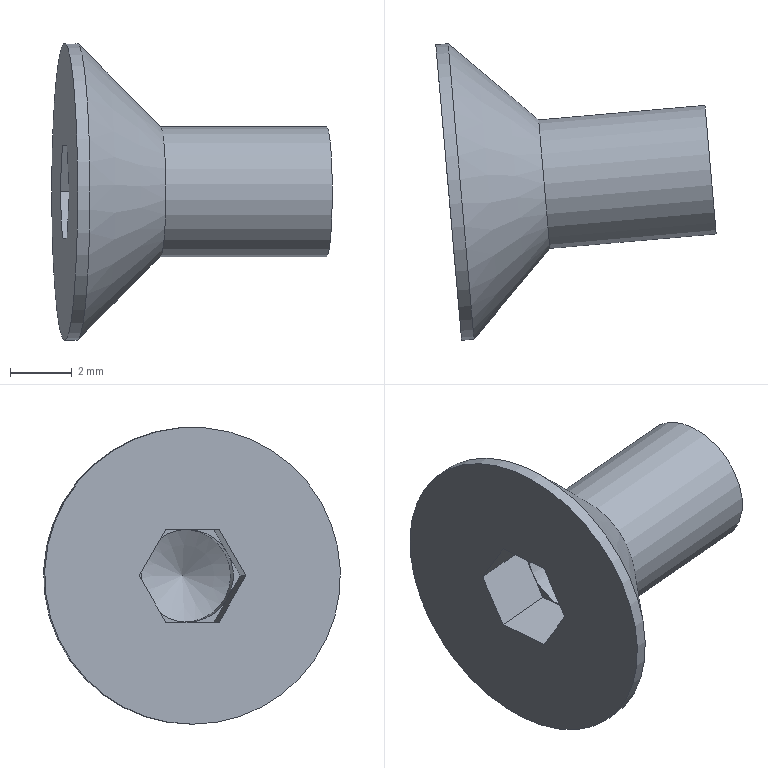Part | NX | features 4 2 | 1 solid | 19 faces | box 9.069 x 9.598 x 9.6 mm | volume 185.183 mm3 | plane 14 | cylinder 3 | cone 2 | commonest cylinder face diameters 3 x1 4.2 x1 9.6 x1
STEP:
#1=CARTESIAN_POINT('',(730.589,495.561,-274.75));
#2=VERTEX_POINT('',#1);
#3=CARTESIAN_POINT('',(730.589,495.561,-273.25));
#4=DIRECTION('',(0.9962,0.08716,0.));
#5=DIRECTION('',(0.,0.,-1.));
#6=AXIS2_PLACEMENT_3D('',#3,#4,#5);
#7=CIRCLE('',#6,1.5);
#8=EDGE_CURVE('',#2,#2,#7,.T.);
#9=ORIENTED_EDGE('',*,*,#8,.F.);
#10=EDGE_LOOP('',(#9));
#11=FACE_BOUND('',#10,.T.);
#12=CARTESIAN_POINT('',(731.452,495.636,-273.25));
#13=VERTEX_POINT('',#12);
#14=VERTEX_LOOP('',#13);
#15=FACE_BOUND('',#14,.T.);
#16=CARTESIAN_POINT('',(731.021,495.599,-273.25));
#17=DIRECTION('',(-0.9962,-0.08716,0.));
#18=DIRECTION('',(0.08716,-0.9962,0.));
#19=AXIS2_PLACEMENT_3D('',#16,#17,#18);
#20=CONICAL_SURFACE('',#19,0.75,1.047);
#21=ADVANCED_FACE('',(#11,#15),#20,.F.);
#22=ORIENTED_EDGE('',*,*,#8,.T.);
#23=EDGE_LOOP('',(#22));
#24=FACE_BOUND('',#23,.T.);
#25=CARTESIAN_POINT('',(729.706,494.18,-274.));
#26=VERTEX_POINT('',#25);
#27=CARTESIAN_POINT('',(729.593,495.474,-274.75));
#28=VERTEX_POINT('',#27);
#29=CARTESIAN_POINT('',(729.593,495.474,-273.25));
#30=DIRECTION('',(0.9962,0.08716,0.));
#31=DIRECTION('',(0.,0.,-1.));
#32=AXIS2_PLACEMENT_3D('',#29,#30,#31);
#33=CIRCLE('',#32,1.5);
#34=EDGE_CURVE('',#26,#28,#33,.T.);
#35=ORIENTED_EDGE('',*,*,#34,.F.);
#36=CARTESIAN_POINT('',(729.706,494.18,-272.5));
#37=VERTEX_POINT('',#36);
#38=CARTESIAN_POINT('',(729.593,495.474,-273.25));
#39=DIRECTION('',(0.9962,0.08716,0.));
#40=DIRECTION('',(0.,0.,-1.));
#41=AXIS2_PLACEMENT_3D('',#38,#39,#40);
#42=CIRCLE('',#41,1.5);
#43=EDGE_CURVE('',#37,#26,#42,.T.);
#44=ORIENTED_EDGE('',*,*,#43,.F.);
#45=CARTESIAN_POINT('',(729.593,495.474,-271.75));
#46=VERTEX_POINT('',#45);
#47=CARTESIAN_POINT('',(729.593,495.474,-273.25));
#48=DIRECTION('',(0.9962,0.08716,0.));
#49=DIRECTION('',(0.,0.,-1.));
#50=AXIS2_PLACEMENT_3D('',#47,#48,#49);
#51=CIRCLE('',#50,1.5);
#52=EDGE_CURVE('',#46,#37,#51,.T.);
#53=ORIENTED_EDGE('',*,*,#52,.F.);
#54=CARTESIAN_POINT('',(729.48,496.768,-272.5));
#55=VERTEX_POINT('',#54);
#56=CARTESIAN_POINT('',(729.593,495.474,-273.25));
#57=DIRECTION('',(0.9962,0.08716,0.));
#58=DIRECTION('',(0.,0.,-1.));
#59=AXIS2_PLACEMENT_3D('',#56,#57,#58);
#60=CIRCLE('',#59,1.5);
#61=EDGE_CURVE('',#55,#46,#60,.T.);
#62=ORIENTED_EDGE('',*,*,#61,.F.);
#63=CARTESIAN_POINT('',(729.48,496.768,-274.));
#64=VERTEX_POINT('',#63);
#65=CARTESIAN_POINT('',(729.593,495.474,-273.25));
#66=DIRECTION('',(0.9962,0.08716,0.));
#67=DIRECTION('',(0.,0.,-1.));
#68=AXIS2_PLACEMENT_3D('',#65,#66,#67);
#69=CIRCLE('',#68,1.5);
#70=EDGE_CURVE('',#64,#55,#69,.T.);
#71=ORIENTED_EDGE('',*,*,#70,.F.);
#72=CARTESIAN_POINT('',(729.593,495.474,-273.25));
#73=DIRECTION('',(0.9962,0.08716,0.));
#74=DIRECTION('',(0.,0.,-1.));
#75=AXIS2_PLACEMENT_3D('',#72,#73,#74);
#76=CIRCLE('',#75,1.5);
#77=EDGE_CURVE('',#28,#64,#76,.T.);
#78=ORIENTED_EDGE('',*,*,#77,.F.);
#79=EDGE_LOOP('',(#35,#44,#53,#62,#71,#78));
#80=FACE_BOUND('',#79,.T.);
#81=CARTESIAN_POINT('',(729.095,495.43,-273.25));
#82=DIRECTION('',(0.9962,0.08716,0.));
#83=DIRECTION('',(-0.08716,0.9962,0.));
#84=AXIS2_PLACEMENT_3D('',#81,#82,#83);
#85=CYLINDRICAL_SURFACE('',#84,1.5);
#86=ADVANCED_FACE('',(#24,#80),#85,.F.);
#87=CARTESIAN_POINT('',(727.999,495.334,-278.05));
#88=VERTEX_POINT('',#87);
#89=CARTESIAN_POINT('',(727.999,495.334,-273.25));
#90=DIRECTION('',(0.9962,0.08716,0.));
#91=DIRECTION('',(0.,0.,-1.));
#92=AXIS2_PLACEMENT_3D('',#89,#90,#91);
#93=CIRCLE('',#92,4.8);
#94=EDGE_CURVE('',#88,#88,#93,.T.);
#95=ORIENTED_EDGE('',*,*,#94,.F.);
#96=EDGE_LOOP('',(#95));
#97=FACE_BOUND('',#96,.T.);
#98=CARTESIAN_POINT('',(727.601,495.299,-278.05));
#99=VERTEX_POINT('',#98);
#100=CARTESIAN_POINT('',(727.601,495.299,-273.25));
#101=DIRECTION('',(0.9962,0.08716,0.));
#102=DIRECTION('',(0.,0.,-1.));
#103=AXIS2_PLACEMENT_3D('',#100,#101,#102);
#104=CIRCLE('',#103,4.8);
#105=EDGE_CURVE('',#99,#99,#104,.T.);
#106=ORIENTED_EDGE('',*,*,#105,.T.);
#107=EDGE_LOOP('',(#106));
#108=FACE_BOUND('',#107,.T.);
#109=CARTESIAN_POINT('',(727.8,495.317,-273.25));
#110=DIRECTION('',(0.9962,0.08716,0.));
#111=DIRECTION('',(-0.08716,0.9962,0.));
#112=AXIS2_PLACEMENT_3D('',#109,#110,#111);
#113=CYLINDRICAL_SURFACE('',#112,4.8);
#114=ADVANCED_FACE('',(#97,#108),#113,.T.);
#115=CARTESIAN_POINT('',(730.689,495.57,-275.35));
#116=VERTEX_POINT('',#115);
#117=CARTESIAN_POINT('',(730.689,495.57,-273.25));
#118=DIRECTION('',(0.9962,0.08716,0.));
#119=DIRECTION('',(0.,0.,-1.));
#120=AXIS2_PLACEMENT_3D('',#117,#118,#119);
#121=CIRCLE('',#120,2.1);
#122=EDGE_CURVE('',#116,#116,#121,.T.);
#123=ORIENTED_EDGE('',*,*,#122,.F.);
#124=EDGE_LOOP('',(#123));
#125=FACE_BOUND('',#124,.T.);
#126=ORIENTED_EDGE('',*,*,#94,.T.);
#127=EDGE_LOOP('',(#126));
#128=FACE_BOUND('',#127,.T.);
#129=CARTESIAN_POINT('',(729.344,495.452,-273.25));
#130=DIRECTION('',(-0.9962,-0.08716,0.));
#131=DIRECTION('',(0.08716,-0.9962,0.));
#132=AXIS2_PLACEMENT_3D('',#129,#130,#131);
#133=CONICAL_SURFACE('',#132,3.45,0.7854);
#134=ADVANCED_FACE('',(#125,#128),#133,.T.);
#135=CARTESIAN_POINT('',(736.068,496.04,-275.35));
#136=VERTEX_POINT('',#135);
#137=CARTESIAN_POINT('',(736.068,496.04,-273.25));
#138=DIRECTION('',(0.9962,0.08716,0.));
#139=DIRECTION('',(0.,0.,-1.));
#140=AXIS2_PLACEMENT_3D('',#137,#138,#139);
#141=CIRCLE('',#140,2.1);
#142=EDGE_CURVE('',#136,#136,#141,.T.);
#143=ORIENTED_EDGE('',*,*,#142,.F.);
#144=EDGE_LOOP('',(#143));
#145=FACE_BOUND('',#144,.T.);
#146=ORIENTED_EDGE('',*,*,#122,.T.);
#147=EDGE_LOOP('',(#146));
#148=FACE_BOUND('',#147,.T.);
#149=CARTESIAN_POINT('',(733.378,495.805,-273.25));
#150=DIRECTION('',(0.9962,0.08716,0.));
#151=DIRECTION('',(-0.08716,0.9962,0.));
#152=AXIS2_PLACEMENT_3D('',#149,#150,#151);
#153=CYLINDRICAL_SURFACE('',#152,2.1);
#154=ADVANCED_FACE('',(#145,#148),#153,.T.);
#155=CARTESIAN_POINT('',(727.676,494.437,-274.75));
#156=VERTEX_POINT('',#155);
#157=CARTESIAN_POINT('',(727.752,493.574,-273.25));
#158=VERTEX_POINT('',#157);
#159=CARTESIAN_POINT('',(727.673,494.469,-274.806));
#160=DIRECTION('',(0.04358,-0.4981,0.866));
#161=VECTOR('',#160,1000.);
#162=LINE('',#159,#161);
#163=EDGE_CURVE('',#156,#158,#162,.T.);
#164=ORIENTED_EDGE('',*,*,#163,.T.);
#165=CARTESIAN_POINT('',(729.744,493.748,-273.25));
#166=VERTEX_POINT('',#165);
#167=CARTESIAN_POINT('',(725.759,493.4,-273.25));
#168=DIRECTION('',(0.9962,0.08716,0.));
#169=VECTOR('',#168,1000.);
#170=LINE('',#167,#169);
#171=EDGE_CURVE('',#158,#166,#170,.T.);
#172=ORIENTED_EDGE('',*,*,#171,.T.);
#173=CARTESIAN_POINT('',(729.744,493.748,-273.25));
#174=DIRECTION('',(-0.04358,0.4981,-0.866));
#175=VECTOR('',#174,1000.);
#176=LINE('',#173,#175);
#177=EDGE_CURVE('',#166,#26,#176,.T.);
#178=ORIENTED_EDGE('',*,*,#177,.T.);
#179=CARTESIAN_POINT('',(729.668,494.611,-274.75));
#180=VERTEX_POINT('',#179);
#181=CARTESIAN_POINT('',(729.744,493.748,-273.25));
#182=DIRECTION('',(-0.04358,0.4981,-0.866));
#183=VECTOR('',#182,1000.);
#184=LINE('',#181,#183);
#185=EDGE_CURVE('',#26,#180,#184,.T.);
#186=ORIENTED_EDGE('',*,*,#185,.T.);
#187=CARTESIAN_POINT('',(725.684,494.262,-274.75));
#188=DIRECTION('',(0.9962,0.08716,0.));
#189=VECTOR('',#188,1000.);
#190=LINE('',#187,#189);
#191=EDGE_CURVE('',#156,#180,#190,.T.);
#192=ORIENTED_EDGE('',*,*,#191,.F.);
#193=EDGE_LOOP('',(#164,#172,#178,#186,#192));
#194=FACE_BOUND('',#193,.T.);
#195=CARTESIAN_POINT('',(725.759,493.4,-273.25));
#196=DIRECTION('',(0.07548,-0.8627,-0.5));
#197=DIRECTION('',(-0.04358,0.4981,-0.866));
#198=AXIS2_PLACEMENT_3D('',#195,#196,#197);
#199=PLANE('',#198);
#200=ADVANCED_FACE('',(#194),#199,.F.);
#201=CARTESIAN_POINT('',(727.525,496.162,-274.75));
#202=VERTEX_POINT('',#201);
#203=CARTESIAN_POINT('',(727.638,494.868,-274.75));
#204=DIRECTION('',(0.08716,-0.9962,0.));
#205=VECTOR('',#204,1000.);
#206=LINE('',#203,#205);
#207=EDGE_CURVE('',#202,#156,#206,.T.);
#208=ORIENTED_EDGE('',*,*,#207,.T.);
#209=ORIENTED_EDGE('',*,*,#191,.T.);
#210=CARTESIAN_POINT('',(729.668,494.611,-274.75));
#211=DIRECTION('',(-0.08716,0.9962,0.));
#212=VECTOR('',#211,1000.);
#213=LINE('',#210,#212);
#214=EDGE_CURVE('',#180,#28,#213,.T.);
#215=ORIENTED_EDGE('',*,*,#214,.T.);
#216=CARTESIAN_POINT('',(729.517,496.336,-274.75));
#217=VERTEX_POINT('',#216);
#218=CARTESIAN_POINT('',(729.668,494.611,-274.75));
#219=DIRECTION('',(-0.08716,0.9962,0.));
#220=VECTOR('',#219,1000.);
#221=LINE('',#218,#220);
#222=EDGE_CURVE('',#28,#217,#221,.T.);
#223=ORIENTED_EDGE('',*,*,#222,.T.);
#224=CARTESIAN_POINT('',(725.533,495.988,-274.75));
#225=DIRECTION('',(0.9962,0.08716,0.));
#226=VECTOR('',#225,1000.);
#227=LINE('',#224,#226);
#228=EDGE_CURVE('',#202,#217,#227,.T.);
#229=ORIENTED_EDGE('',*,*,#228,.F.);
#230=EDGE_LOOP('',(#208,#209,#215,#223,#229));
#231=FACE_BOUND('',#230,.T.);
#232=CARTESIAN_POINT('',(725.684,494.262,-274.75));
#233=DIRECTION('',(0.,0.,-1.));
#234=DIRECTION('',(-0.9962,-0.08716,0.));
#235=AXIS2_PLACEMENT_3D('',#232,#233,#234);
#236=PLANE('',#235);
#237=ADVANCED_FACE('',(#231),#236,.F.);
#238=CARTESIAN_POINT('',(727.676,494.437,-271.75));
#239=VERTEX_POINT('',#238);
#240=CARTESIAN_POINT('',(727.754,493.542,-273.306));
#241=DIRECTION('',(-0.04358,0.4981,0.866));
#242=VECTOR('',#241,1000.);
#243=LINE('',#240,#242);
#244=EDGE_CURVE('',#158,#239,#243,.T.);
#245=ORIENTED_EDGE('',*,*,#244,.T.);
#246=CARTESIAN_POINT('',(729.668,494.611,-271.75));
#247=VERTEX_POINT('',#246);
#248=CARTESIAN_POINT('',(725.684,494.262,-271.75));
#249=DIRECTION('',(0.9962,0.08716,0.));
#250=VECTOR('',#249,1000.);
#251=LINE('',#248,#250);
#252=EDGE_CURVE('',#239,#247,#251,.T.);
#253=ORIENTED_EDGE('',*,*,#252,.T.);
#254=CARTESIAN_POINT('',(729.668,494.611,-271.75));
#255=DIRECTION('',(0.04358,-0.4981,-0.866));
#256=VECTOR('',#255,1000.);
#257=LINE('',#254,#256);
#258=EDGE_CURVE('',#247,#37,#257,.T.);
#259=ORIENTED_EDGE('',*,*,#258,.T.);
#260=CARTESIAN_POINT('',(729.668,494.611,-271.75));
#261=DIRECTION('',(0.04358,-0.4981,-0.866));
#262=VECTOR('',#261,1000.);
#263=LINE('',#260,#262);
#264=EDGE_CURVE('',#37,#166,#263,.T.);
#265=ORIENTED_EDGE('',*,*,#264,.T.);
#266=ORIENTED_EDGE('',*,*,#171,.F.);
#267=EDGE_LOOP('',(#245,#253,#259,#265,#266));
#268=FACE_BOUND('',#267,.T.);
#269=CARTESIAN_POINT('',(725.684,494.262,-271.75));
#270=DIRECTION('',(0.07548,-0.8627,0.5));
#271=DIRECTION('',(0.04358,-0.4981,-0.866));
#272=AXIS2_PLACEMENT_3D('',#269,#270,#271);
#273=PLANE('',#272);
#274=ADVANCED_FACE('',(#268),#273,.F.);
#275=CARTESIAN_POINT('',(727.45,497.025,-273.25));
#276=VERTEX_POINT('',#275);
#277=CARTESIAN_POINT('',(727.566,495.698,-275.556));
#278=DIRECTION('',(0.04358,-0.4981,-0.866));
#279=VECTOR('',#278,1000.);
#280=LINE('',#277,#279);
#281=EDGE_CURVE('',#276,#202,#280,.T.);
#282=ORIENTED_EDGE('',*,*,#281,.T.);
#283=ORIENTED_EDGE('',*,*,#228,.T.);
#284=CARTESIAN_POINT('',(729.517,496.336,-274.75));
#285=DIRECTION('',(-0.04358,0.4981,0.866));
#286=VECTOR('',#285,1000.);
#287=LINE('',#284,#286);
#288=EDGE_CURVE('',#217,#64,#287,.T.);
#289=ORIENTED_EDGE('',*,*,#288,.T.);
#290=CARTESIAN_POINT('',(729.442,497.199,-273.25));
#291=VERTEX_POINT('',#290);
#292=CARTESIAN_POINT('',(729.517,496.336,-274.75));
#293=DIRECTION('',(-0.04358,0.4981,0.866));
#294=VECTOR('',#293,1000.);
#295=LINE('',#292,#294);
#296=EDGE_CURVE('',#64,#291,#295,.T.);
#297=ORIENTED_EDGE('',*,*,#296,.T.);
#298=CARTESIAN_POINT('',(725.457,496.85,-273.25));
#299=DIRECTION('',(0.9962,0.08716,0.));
#300=VECTOR('',#299,1000.);
#301=LINE('',#298,#300);
#302=EDGE_CURVE('',#276,#291,#301,.T.);
#303=ORIENTED_EDGE('',*,*,#302,.F.);
#304=EDGE_LOOP('',(#282,#283,#289,#297,#303));
#305=FACE_BOUND('',#304,.T.);
#306=CARTESIAN_POINT('',(725.533,495.988,-274.75));
#307=DIRECTION('',(-0.07548,0.8627,-0.5));
#308=DIRECTION('',(-0.04358,0.4981,0.866));
#309=AXIS2_PLACEMENT_3D('',#306,#307,#308);
#310=PLANE('',#309);
#311=ADVANCED_FACE('',(#305),#310,.F.);
#312=ORIENTED_EDGE('',*,*,#61,.T.);
#313=CARTESIAN_POINT('',(729.517,496.336,-271.75));
#314=VERTEX_POINT('',#313);
#315=CARTESIAN_POINT('',(729.517,496.336,-271.75));
#316=DIRECTION('',(0.08716,-0.9962,0.));
#317=VECTOR('',#316,1000.);
#318=LINE('',#315,#317);
#319=EDGE_CURVE('',#314,#46,#318,.T.);
#320=ORIENTED_EDGE('',*,*,#319,.F.);
#321=CARTESIAN_POINT('',(729.442,497.199,-273.25));
#322=DIRECTION('',(0.04358,-0.4981,0.866));
#323=VECTOR('',#322,1000.);
#324=LINE('',#321,#323);
#325=EDGE_CURVE('',#55,#314,#324,.T.);
#326=ORIENTED_EDGE('',*,*,#325,.F.);
#327=EDGE_LOOP('',(#312,#320,#326));
#328=FACE_BOUND('',#327,.T.);
#329=CARTESIAN_POINT('',(729.593,495.474,-273.25));
#330=DIRECTION('',(-0.9962,-0.08716,0.));
#331=DIRECTION('',(0.08716,-0.9962,0.));
#332=AXIS2_PLACEMENT_3D('',#329,#330,#331);
#333=PLANE('',#332);
#334=ADVANCED_FACE('',(#328),#333,.T.);
#335=ORIENTED_EDGE('',*,*,#52,.T.);
#336=ORIENTED_EDGE('',*,*,#258,.F.);
#337=CARTESIAN_POINT('',(729.517,496.336,-271.75));
#338=DIRECTION('',(0.08716,-0.9962,0.));
#339=VECTOR('',#338,1000.);
#340=LINE('',#337,#339);
#341=EDGE_CURVE('',#46,#247,#340,.T.);
#342=ORIENTED_EDGE('',*,*,#341,.F.);
#343=EDGE_LOOP('',(#335,#336,#342));
#344=FACE_BOUND('',#343,.T.);
#345=CARTESIAN_POINT('',(729.593,495.474,-273.25));
#346=DIRECTION('',(-0.9962,-0.08716,0.));
#347=DIRECTION('',(0.08716,-0.9962,0.));
#348=AXIS2_PLACEMENT_3D('',#345,#346,#347);
#349=PLANE('',#348);
#350=ADVANCED_FACE('',(#344),#349,.T.);
#351=ORIENTED_EDGE('',*,*,#43,.T.);
#352=ORIENTED_EDGE('',*,*,#177,.F.);
#353=ORIENTED_EDGE('',*,*,#264,.F.);
#354=EDGE_LOOP('',(#351,#352,#353));
#355=FACE_BOUND('',#354,.T.);
#356=CARTESIAN_POINT('',(729.593,495.474,-273.25));
#357=DIRECTION('',(-0.9962,-0.08716,0.));
#358=DIRECTION('',(0.08716,-0.9962,0.));
#359=AXIS2_PLACEMENT_3D('',#356,#357,#358);
#360=PLANE('',#359);
#361=ADVANCED_FACE('',(#355),#360,.T.);
#362=ORIENTED_EDGE('',*,*,#34,.T.);
#363=ORIENTED_EDGE('',*,*,#214,.F.);
#364=ORIENTED_EDGE('',*,*,#185,.F.);
#365=EDGE_LOOP('',(#362,#363,#364));
#366=FACE_BOUND('',#365,.T.);
#367=CARTESIAN_POINT('',(729.593,495.474,-273.25));
#368=DIRECTION('',(-0.9962,-0.08716,0.));
#369=DIRECTION('',(0.08716,-0.9962,0.));
#370=AXIS2_PLACEMENT_3D('',#367,#368,#369);
#371=PLANE('',#370);
#372=ADVANCED_FACE('',(#366),#371,.T.);
#373=ORIENTED_EDGE('',*,*,#77,.T.);
#374=ORIENTED_EDGE('',*,*,#288,.F.);
#375=ORIENTED_EDGE('',*,*,#222,.F.);
#376=EDGE_LOOP('',(#373,#374,#375));
#377=FACE_BOUND('',#376,.T.);
#378=CARTESIAN_POINT('',(729.593,495.474,-273.25));
#379=DIRECTION('',(-0.9962,-0.08716,0.));
#380=DIRECTION('',(0.08716,-0.9962,0.));
#381=AXIS2_PLACEMENT_3D('',#378,#379,#380);
#382=PLANE('',#381);
#383=ADVANCED_FACE('',(#377),#382,.T.);
#384=ORIENTED_EDGE('',*,*,#70,.T.);
#385=CARTESIAN_POINT('',(729.442,497.199,-273.25));
#386=DIRECTION('',(0.04358,-0.4981,0.866));
#387=VECTOR('',#386,1000.);
#388=LINE('',#385,#387);
#389=EDGE_CURVE('',#291,#55,#388,.T.);
#390=ORIENTED_EDGE('',*,*,#389,.F.);
#391=ORIENTED_EDGE('',*,*,#296,.F.);
#392=EDGE_LOOP('',(#384,#390,#391));
#393=FACE_BOUND('',#392,.T.);
#394=CARTESIAN_POINT('',(729.593,495.474,-273.25));
#395=DIRECTION('',(-0.9962,-0.08716,0.));
#396=DIRECTION('',(0.08716,-0.9962,0.));
#397=AXIS2_PLACEMENT_3D('',#394,#395,#396);
#398=PLANE('',#397);
#399=ADVANCED_FACE('',(#393),#398,.T.);
#400=CARTESIAN_POINT('',(727.525,496.162,-271.75));
#401=VERTEX_POINT('',#400);
#402=CARTESIAN_POINT('',(727.563,495.731,-271.75));
#403=DIRECTION('',(-0.08716,0.9962,0.));
#404=VECTOR('',#403,1000.);
#405=LINE('',#402,#404);
#406=EDGE_CURVE('',#239,#401,#405,.T.);
#407=ORIENTED_EDGE('',*,*,#406,.T.);
#408=CARTESIAN_POINT('',(725.533,495.988,-271.75));
#409=DIRECTION('',(0.9962,0.08716,0.));
#410=VECTOR('',#409,1000.);
#411=LINE('',#408,#410);
#412=EDGE_CURVE('',#401,#314,#411,.T.);
#413=ORIENTED_EDGE('',*,*,#412,.T.);
#414=ORIENTED_EDGE('',*,*,#319,.T.);
#415=ORIENTED_EDGE('',*,*,#341,.T.);
#416=ORIENTED_EDGE('',*,*,#252,.F.);
#417=EDGE_LOOP('',(#407,#413,#414,#415,#416));
#418=FACE_BOUND('',#417,.T.);
#419=CARTESIAN_POINT('',(725.533,495.988,-271.75));
#420=DIRECTION('',(0.,0.,1.));
#421=DIRECTION('',(0.9962,0.08716,0.));
#422=AXIS2_PLACEMENT_3D('',#419,#420,#421);
#423=PLANE('',#422);
#424=ADVANCED_FACE('',(#418),#423,.F.);
#425=CARTESIAN_POINT('',(727.409,497.489,-274.056));
#426=DIRECTION('',(-0.04358,0.4981,-0.866));
#427=VECTOR('',#426,1000.);
#428=LINE('',#425,#427);
#429=EDGE_CURVE('',#401,#276,#428,.T.);
#430=ORIENTED_EDGE('',*,*,#429,.T.);
#431=ORIENTED_EDGE('',*,*,#302,.T.);
#432=ORIENTED_EDGE('',*,*,#389,.T.);
#433=ORIENTED_EDGE('',*,*,#325,.T.);
#434=ORIENTED_EDGE('',*,*,#412,.F.);
#435=EDGE_LOOP('',(#430,#431,#432,#433,#434));
#436=FACE_BOUND('',#435,.T.);
#437=CARTESIAN_POINT('',(725.457,496.85,-273.25));
#438=DIRECTION('',(-0.07548,0.8627,0.5));
#439=DIRECTION('',(0.04358,-0.4981,0.866));
#440=AXIS2_PLACEMENT_3D('',#437,#438,#439);
#441=PLANE('',#440);
#442=ADVANCED_FACE('',(#436),#441,.F.);
#443=ORIENTED_EDGE('',*,*,#142,.T.);
#444=EDGE_LOOP('',(#443));
#445=FACE_BOUND('',#444,.T.);
#446=CARTESIAN_POINT('',(736.068,496.04,-274.3));
#447=DIRECTION('',(0.9962,0.08716,0.));
#448=DIRECTION('',(-0.08716,0.9962,0.));
#449=AXIS2_PLACEMENT_3D('',#446,#447,#448);
#450=PLANE('',#449);
#451=ADVANCED_FACE('',(#445),#450,.T.);
#452=ORIENTED_EDGE('',*,*,#429,.F.);
#453=ORIENTED_EDGE('',*,*,#406,.F.);
#454=ORIENTED_EDGE('',*,*,#244,.F.);
#455=ORIENTED_EDGE('',*,*,#163,.F.);
#456=ORIENTED_EDGE('',*,*,#207,.F.);
#457=ORIENTED_EDGE('',*,*,#281,.F.);
#458=EDGE_LOOP('',(#452,#453,#454,#455,#456,#457));
#459=FACE_BOUND('',#458,.T.);
#460=ORIENTED_EDGE('',*,*,#105,.F.);
#461=EDGE_LOOP('',(#460));
#462=FACE_BOUND('',#461,.T.);
#463=CARTESIAN_POINT('',(727.601,495.299,-276.4));
#464=DIRECTION('',(-0.9962,-0.08716,0.));
#465=DIRECTION('',(0.08716,-0.9962,0.));
#466=AXIS2_PLACEMENT_3D('',#463,#464,#465);
#467=PLANE('',#466);
#468=ADVANCED_FACE('',(#459,#462),#467,.T.);
#469=CLOSED_SHELL('',(#21,#86,#114,#134,#154,#200,#237,#274,#311,#334,#350,#361,#372,#383,#399,#424,#442,#451,#468));
#470=MANIFOLD_SOLID_BREP('',#469);
#471=(LENGTH_UNIT()NAMED_UNIT(*)SI_UNIT(.MILLI.,.METRE.));
#472=UNCERTAINTY_MEASURE_WITH_UNIT(LENGTH_MEASURE(0.00001),#471,'','');
#473=(NAMED_UNIT(*)PLANE_ANGLE_UNIT()SI_UNIT($,.RADIAN.));
#474=(NAMED_UNIT(*)SI_UNIT($,.STERADIAN.)SOLID_ANGLE_UNIT());
#475=(GEOMETRIC_REPRESENTATION_CONTEXT(3)GLOBAL_UNCERTAINTY_ASSIGNED_CONTEXT((#472))GLOBAL_UNIT_ASSIGNED_CONTEXT((#471,#473,#474))REPRESENTATION_CONTEXT('',''));
#476=ADVANCED_BREP_SHAPE_REPRESENTATION('',(#470),#475);